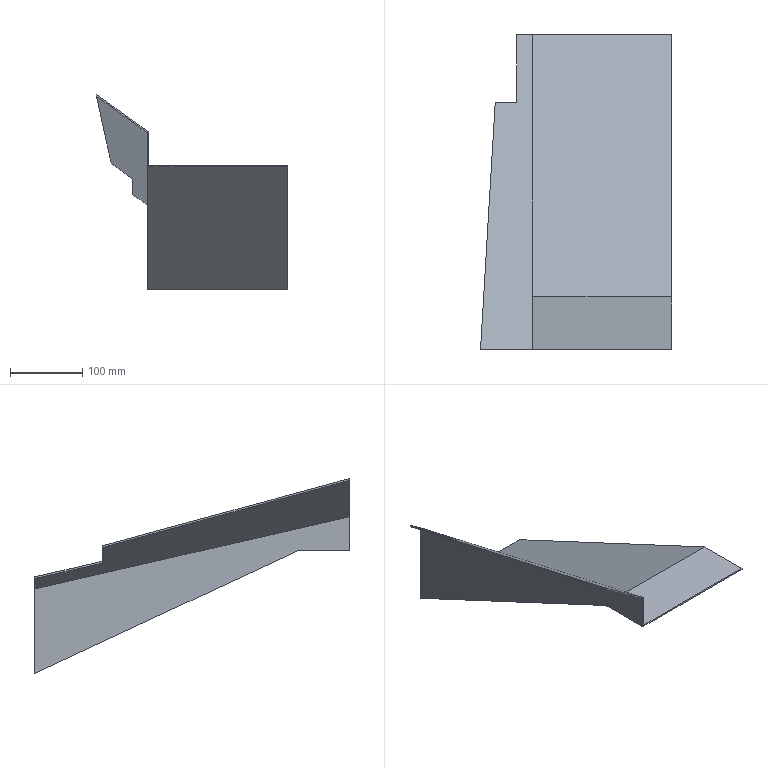Part | NX | features solid 2 | 1 solid | 14 faces | box 265.119 x 436.993 x 270.643 mm | volume 301955 mm3 | plane 13 | spline 1
STEP:
#1=CARTESIAN_POINT('',(815.34,325.702,-147.77));
#2=VERTEX_POINT('',#1);
#3=CARTESIAN_POINT('',(785.34,325.702,-126.218));
#4=VERTEX_POINT('',#3);
#5=CARTESIAN_POINT('',(723.013,325.702,-81.441));
#6=DIRECTION('',(0.8121,0.,-0.5835));
#7=VECTOR('',#6,1000.);
#8=LINE('',#5,#7);
#9=EDGE_CURVE('',#2,#4,#8,.F.);
#10=ORIENTED_EDGE('',*,*,#9,.F.);
#11=CARTESIAN_POINT('',(815.34,325.702,-150.275));
#12=VERTEX_POINT('',#11);
#13=CARTESIAN_POINT('',(815.34,325.702,-80.177));
#14=DIRECTION('',(0.,0.,-1.));
#15=VECTOR('',#14,1000.);
#16=LINE('',#13,#15);
#17=EDGE_CURVE('',#2,#12,#16,.T.);
#18=ORIENTED_EDGE('',*,*,#17,.T.);
#19=CARTESIAN_POINT('',(785.34,325.702,-128.723));
#20=VERTEX_POINT('',#19);
#21=CARTESIAN_POINT('',(721.826,325.702,-83.094));
#22=DIRECTION('',(0.8121,0.,-0.5835));
#23=VECTOR('',#22,1000.);
#24=LINE('',#21,#23);
#25=EDGE_CURVE('',#20,#12,#24,.T.);
#26=ORIENTED_EDGE('',*,*,#25,.F.);
#27=CARTESIAN_POINT('',(785.34,325.702,-80.177));
#28=DIRECTION('',(0.,0.,-1.));
#29=VECTOR('',#28,1000.);
#30=LINE('',#27,#29);
#31=EDGE_CURVE('',#4,#20,#30,.T.);
#32=ORIENTED_EDGE('',*,*,#31,.F.);
#33=EDGE_LOOP('',(#10,#18,#26,#32));
#34=FACE_BOUND('',#33,.T.);
#35=CARTESIAN_POINT('',(772.317,325.702,-80.177));
#36=DIRECTION('',(0.,-1.,0.));
#37=DIRECTION('',(0.,0.,-1.));
#38=AXIS2_PLACEMENT_3D('',#35,#36,#37);
#39=PLANE('',#38);
#40=ADVANCED_FACE('',(#34),#39,.F.);
#41=CARTESIAN_POINT('',(764.881,-17.,-32.884));
#42=VERTEX_POINT('',#41);
#43=CARTESIAN_POINT('',(837.317,-17.,-84.922));
#44=VERTEX_POINT('',#43);
#45=CARTESIAN_POINT('',(764.881,-17.,-32.884));
#46=CARTESIAN_POINT('',(789.026,-17.,-50.23));
#47=CARTESIAN_POINT('',(813.171,-17.,-67.576));
#48=CARTESIAN_POINT('',(837.317,-17.,-84.922));
#49=B_SPLINE_CURVE_WITH_KNOTS('',3,(#45,#46,#47,#48),.UNSPECIFIED.,.F.,.F.,(4,4),(-0.01905,0.07014),.UNSPECIFIED.);
#50=EDGE_CURVE('',#42,#44,#49,.T.);
#51=ORIENTED_EDGE('',*,*,#50,.F.);
#52=CARTESIAN_POINT('',(764.881,-17.,-35.389));
#53=VERTEX_POINT('',#52);
#54=CARTESIAN_POINT('',(764.881,-17.,-33.012));
#55=DIRECTION('',(0.,0.,1.));
#56=VECTOR('',#55,1000.);
#57=LINE('',#54,#56);
#58=EDGE_CURVE('',#42,#53,#57,.F.);
#59=ORIENTED_EDGE('',*,*,#58,.T.);
#60=CARTESIAN_POINT('',(835.317,-17.,-85.99));
#61=VERTEX_POINT('',#60);
#62=CARTESIAN_POINT('',(764.881,-17.,-35.389));
#63=CARTESIAN_POINT('',(788.359,-17.,-52.256));
#64=CARTESIAN_POINT('',(811.838,-17.,-69.123));
#65=CARTESIAN_POINT('',(835.317,-17.,-85.99));
#66=B_SPLINE_CURVE_WITH_KNOTS('',3,(#62,#63,#64,#65),.UNSPECIFIED.,.F.,.F.,(4,4),(-0.01764,0.06909),.UNSPECIFIED.);
#67=EDGE_CURVE('',#53,#61,#66,.T.);
#68=ORIENTED_EDGE('',*,*,#67,.T.);
#69=CARTESIAN_POINT('',(835.317,-17.,-133.495));
#70=VERTEX_POINT('',#69);
#71=CARTESIAN_POINT('',(835.317,-17.,-107.104));
#72=DIRECTION('',(0.,0.,1.));
#73=VECTOR('',#72,1000.);
#74=LINE('',#71,#73);
#75=EDGE_CURVE('',#70,#61,#74,.T.);
#76=ORIENTED_EDGE('',*,*,#75,.F.);
#77=CARTESIAN_POINT('',(1030.,-17.,-133.495));
#78=VERTEX_POINT('',#77);
#79=CARTESIAN_POINT('',(835.317,-17.,-133.495));
#80=CARTESIAN_POINT('',(900.211,-17.,-133.495));
#81=CARTESIAN_POINT('',(965.106,-17.,-133.495));
#82=CARTESIAN_POINT('',(1030.,-17.,-133.495));
#83=B_SPLINE_CURVE_WITH_KNOTS('',3,(#79,#80,#81,#82),.UNSPECIFIED.,.F.,.F.,(4,4),(0.,0.1947),.UNSPECIFIED.);
#84=EDGE_CURVE('',#70,#78,#83,.T.);
#85=ORIENTED_EDGE('',*,*,#84,.T.);
#86=CARTESIAN_POINT('',(1030.,-17.,-131.495));
#87=VERTEX_POINT('',#86);
#88=CARTESIAN_POINT('',(1030.,-17.,-132.495));
#89=DIRECTION('',(0.,0.,1.));
#90=VECTOR('',#89,1000.);
#91=LINE('',#88,#90);
#92=EDGE_CURVE('',#78,#87,#91,.T.);
#93=ORIENTED_EDGE('',*,*,#92,.T.);
#94=CARTESIAN_POINT('',(837.317,-17.,-131.495));
#95=VERTEX_POINT('',#94);
#96=CARTESIAN_POINT('',(837.317,-17.,-131.495));
#97=CARTESIAN_POINT('',(901.544,-17.,-131.495));
#98=CARTESIAN_POINT('',(965.772,-17.,-131.495));
#99=CARTESIAN_POINT('',(1030.,-17.,-131.495));
#100=B_SPLINE_CURVE_WITH_KNOTS('',3,(#96,#97,#98,#99),.UNSPECIFIED.,.F.,.F.,(4,4),(0.,0.1927),.UNSPECIFIED.);
#101=EDGE_CURVE('',#95,#87,#100,.T.);
#102=ORIENTED_EDGE('',*,*,#101,.F.);
#103=CARTESIAN_POINT('',(837.317,-17.,-105.57));
#104=DIRECTION('',(0.,0.,1.));
#105=VECTOR('',#104,1000.);
#106=LINE('',#103,#105);
#107=EDGE_CURVE('',#44,#95,#106,.F.);
#108=ORIENTED_EDGE('',*,*,#107,.F.);
#109=EDGE_LOOP('',(#51,#59,#68,#76,#85,#93,#102,#108));
#110=FACE_BOUND('',#109,.T.);
#111=CARTESIAN_POINT('',(1030.,-17.,-139.629));
#112=CARTESIAN_POINT('',(1030.,-17.,-42.536));
#113=CARTESIAN_POINT('',(1017.249,-17.,-139.629));
#114=CARTESIAN_POINT('',(1017.249,-17.,-42.536));
#115=CARTESIAN_POINT('',(991.747,-17.,-139.629));
#116=CARTESIAN_POINT('',(991.747,-17.,-42.536));
#117=CARTESIAN_POINT('',(959.87,-17.,-139.629));
#118=CARTESIAN_POINT('',(959.87,-17.,-42.536));
#119=CARTESIAN_POINT('',(934.368,-17.,-139.629));
#120=CARTESIAN_POINT('',(934.368,-17.,-42.536));
#121=CARTESIAN_POINT('',(915.241,-17.,-139.629));
#122=CARTESIAN_POINT('',(915.241,-17.,-42.536));
#123=CARTESIAN_POINT('',(896.115,-17.,-139.63));
#124=CARTESIAN_POINT('',(896.115,-17.,-42.537));
#125=CARTESIAN_POINT('',(880.175,-17.,-139.627));
#126=CARTESIAN_POINT('',(880.175,-17.,-42.533));
#127=CARTESIAN_POINT('',(869.02,-17.,-139.633));
#128=CARTESIAN_POINT('',(869.02,-17.,-42.539));
#129=CARTESIAN_POINT('',(862.641,-17.,-139.623));
#130=CARTESIAN_POINT('',(862.641,-17.,-42.53));
#131=CARTESIAN_POINT('',(857.869,-17.,-139.653));
#132=CARTESIAN_POINT('',(857.869,-17.,-42.559));
#133=CARTESIAN_POINT('',(853.037,-17.,-139.488));
#134=CARTESIAN_POINT('',(853.037,-17.,-42.395));
#135=CARTESIAN_POINT('',(848.214,-17.,-139.341));
#136=CARTESIAN_POINT('',(848.214,-17.,-42.248));
#137=CARTESIAN_POINT('',(843.577,-17.,-139.83));
#138=CARTESIAN_POINT('',(843.577,-17.,-42.737));
#139=CARTESIAN_POINT('',(839.137,-17.,-141.121));
#140=CARTESIAN_POINT('',(839.137,-17.,-44.028));
#141=CARTESIAN_POINT('',(834.715,-17.,-142.775));
#142=CARTESIAN_POINT('',(834.715,-17.,-45.682));
#143=CARTESIAN_POINT('',(828.593,-17.,-144.624));
#144=CARTESIAN_POINT('',(828.593,-17.,-47.531));
#145=CARTESIAN_POINT('',(820.431,-17.,-144.906));
#146=CARTESIAN_POINT('',(820.431,-17.,-47.812));
#147=CARTESIAN_POINT('',(812.873,-17.,-142.36));
#148=CARTESIAN_POINT('',(812.873,-17.,-45.267));
#149=CARTESIAN_POINT('',(807.015,-17.,-140.172));
#150=CARTESIAN_POINT('',(807.015,-17.,-43.079));
#151=CARTESIAN_POINT('',(801.031,-17.,-138.263));
#152=CARTESIAN_POINT('',(801.031,-17.,-41.17));
#153=CARTESIAN_POINT('',(793.243,-17.,-136.384));
#154=CARTESIAN_POINT('',(793.243,-17.,-39.291));
#155=CARTESIAN_POINT('',(784.909,-17.,-131.641));
#156=CARTESIAN_POINT('',(784.909,-17.,-34.548));
#157=CARTESIAN_POINT('',(778.905,-17.,-123.694));
#158=CARTESIAN_POINT('',(778.905,-17.,-26.601));
#159=CARTESIAN_POINT('',(775.672,-17.,-116.308));
#160=CARTESIAN_POINT('',(775.672,-17.,-19.215));
#161=CARTESIAN_POINT('',(773.734,-17.,-110.553));
#162=CARTESIAN_POINT('',(773.734,-17.,-13.459));
#163=CARTESIAN_POINT('',(772.653,-17.,-106.122));
#164=CARTESIAN_POINT('',(772.653,-17.,-9.029));
#165=CARTESIAN_POINT('',(772.039,-17.,-101.297));
#166=CARTESIAN_POINT('',(772.039,-17.,-4.204));
#167=CARTESIAN_POINT('',(771.795,-17.,-94.179));
#168=CARTESIAN_POINT('',(771.795,-17.,2.914));
#169=CARTESIAN_POINT('',(771.535,-17.,-86.911));
#170=CARTESIAN_POINT('',(771.535,-17.,10.182));
#171=CARTESIAN_POINT('',(768.627,-17.,-82.777));
#172=CARTESIAN_POINT('',(768.627,-17.,14.316));
#173=CARTESIAN_POINT('',(766.237,-17.,-81.837));
#174=CARTESIAN_POINT('',(766.237,-17.,15.257));
#175=CARTESIAN_POINT('',(764.881,-17.,-81.558));
#176=CARTESIAN_POINT('',(764.881,-17.,15.535));
#177=B_SPLINE_SURFACE_WITH_KNOTS('',3,1,((#111,#112),(#113,#114),(#115,#116),(#117,#118),(#119,#120),(#121,#122),(#123,#124),(#125,#126),(#127,#128),(#129,#130),(#131,#132),(#133,#134),(#135,#136),(#137,#138),(#139,#140),(#141,#142),(#143,#144),(#145,#146),(#147,#148),(#149,#150),(#151,#152),(#153,#154),(#155,#156),(#157,#158),(#159,#160),(#161,#162),(#163,#164),(#165,#166),(#167,#168),(#169,#170),(#171,#172),(#173,#174),(#175,#176)),.SURF_OF_LINEAR_EXTRUSION.,.F.,.F.,.F.,(4,1,1,1,1,1,1,1,1,1,1,1,1,1,1,1,1,1,1,1,1,1,1,1,1,1,1,1,1,1,4),(2,2),(-1.184,-0.9175,-0.6509,-0.5176,-0.3843,-0.251,-0.1177,-0.051,-0.01768,0.01565,0.04898,0.08231,0.1156,0.149,0.1823,0.2156,0.2823,0.3489,0.3823,0.4156,0.4822,0.5489,0.6155,0.6822,0.7155,0.7489,0.7822,0.8155,0.8822,0.9155,0.9488),(0.,1.),.UNSPECIFIED.);
#178=ADVANCED_FACE('',(#110),#177,.F.);
#179=ORIENTED_EDGE('',*,*,#50,.T.);
#180=CARTESIAN_POINT('',(837.317,419.993,-185.194));
#181=VERTEX_POINT('',#180);
#182=CARTESIAN_POINT('',(837.317,418.909,-184.945));
#183=DIRECTION('',(0.,0.9747,-0.2236));
#184=VECTOR('',#183,1000.);
#185=LINE('',#182,#184);
#186=EDGE_CURVE('',#181,#44,#185,.F.);
#187=ORIENTED_EDGE('',*,*,#186,.F.);
#188=CARTESIAN_POINT('',(815.34,419.993,-169.406));
#189=VERTEX_POINT('',#188);
#190=CARTESIAN_POINT('',(792.078,419.993,-152.694));
#191=DIRECTION('',(-0.8121,0.,0.5835));
#192=VECTOR('',#191,1000.);
#193=LINE('',#190,#192);
#194=EDGE_CURVE('',#181,#189,#193,.T.);
#195=ORIENTED_EDGE('',*,*,#194,.T.);
#196=CARTESIAN_POINT('',(815.34,349.955,-153.335));
#197=DIRECTION('',(0.,0.9747,-0.2236));
#198=VECTOR('',#197,1000.);
#199=LINE('',#196,#198);
#200=EDGE_CURVE('',#189,#2,#199,.F.);
#201=ORIENTED_EDGE('',*,*,#200,.T.);
#202=ORIENTED_EDGE('',*,*,#9,.T.);
#203=CARTESIAN_POINT('',(790.938,419.454,-151.751));
#204=DIRECTION('',(-0.05751,-0.9633,0.2623));
#205=VECTOR('',#204,1000.);
#206=LINE('',#203,#205);
#207=EDGE_CURVE('',#42,#4,#206,.F.);
#208=ORIENTED_EDGE('',*,*,#207,.F.);
#209=EDGE_LOOP('',(#179,#187,#195,#201,#202,#208));
#210=FACE_BOUND('',#209,.T.);
#211=CARTESIAN_POINT('',(710.723,438.733,-98.548));
#212=DIRECTION('',(0.5736,0.1832,0.7984));
#213=DIRECTION('',(-0.1552,0.9813,-0.1137));
#214=AXIS2_PLACEMENT_3D('',#211,#212,#213);
#215=PLANE('',#214);
#216=ADVANCED_FACE('',(#210),#215,.T.);
#217=ORIENTED_EDGE('',*,*,#25,.T.);
#218=CARTESIAN_POINT('',(815.34,419.993,-171.911));
#219=VERTEX_POINT('',#218);
#220=CARTESIAN_POINT('',(815.34,421.804,-172.326));
#221=DIRECTION('',(0.,-0.9747,0.2236));
#222=VECTOR('',#221,1000.);
#223=LINE('',#220,#222);
#224=EDGE_CURVE('',#219,#12,#223,.T.);
#225=ORIENTED_EDGE('',*,*,#224,.F.);
#226=CARTESIAN_POINT('',(835.317,419.993,-186.262));
#227=VERTEX_POINT('',#226);
#228=CARTESIAN_POINT('',(790.891,419.993,-154.346));
#229=DIRECTION('',(0.8121,0.,-0.5835));
#230=VECTOR('',#229,1000.);
#231=LINE('',#228,#230);
#232=EDGE_CURVE('',#219,#227,#231,.T.);
#233=ORIENTED_EDGE('',*,*,#232,.T.);
#234=CARTESIAN_POINT('',(835.317,322.751,-163.949));
#235=DIRECTION('',(0.,-0.9747,0.2236));
#236=VECTOR('',#235,1000.);
#237=LINE('',#234,#236);
#238=EDGE_CURVE('',#227,#61,#237,.T.);
#239=ORIENTED_EDGE('',*,*,#238,.T.);
#240=ORIENTED_EDGE('',*,*,#67,.F.);
#241=CARTESIAN_POINT('',(790.9,418.821,-154.084));
#242=DIRECTION('',(-0.05751,-0.9633,0.2623));
#243=VECTOR('',#242,1000.);
#244=LINE('',#241,#243);
#245=EDGE_CURVE('',#20,#53,#244,.T.);
#246=ORIENTED_EDGE('',*,*,#245,.F.);
#247=EDGE_LOOP('',(#217,#225,#233,#239,#240,#246));
#248=FACE_BOUND('',#247,.T.);
#249=CARTESIAN_POINT('',(709.576,438.367,-100.145));
#250=DIRECTION('',(0.5736,0.1832,0.7984));
#251=DIRECTION('',(-0.1552,0.9813,-0.1137));
#252=AXIS2_PLACEMENT_3D('',#249,#250,#251);
#253=PLANE('',#252);
#254=ADVANCED_FACE('',(#248),#253,.F.);
#255=CARTESIAN_POINT('',(1030.,419.993,-301.319));
#256=VERTEX_POINT('',#255);
#257=CARTESIAN_POINT('',(1030.,55.804,-131.495));
#258=VERTEX_POINT('',#257);
#259=CARTESIAN_POINT('',(1030.,442.654,-311.886));
#260=DIRECTION('',(0.,-0.9063,0.4226));
#261=VECTOR('',#260,1000.);
#262=LINE('',#259,#261);
#263=EDGE_CURVE('',#256,#258,#262,.T.);
#264=ORIENTED_EDGE('',*,*,#263,.F.);
#265=CARTESIAN_POINT('',(837.317,419.993,-301.319));
#266=VERTEX_POINT('',#265);
#267=CARTESIAN_POINT('',(747.317,419.993,-301.319));
#268=DIRECTION('',(1.,0.,0.));
#269=VECTOR('',#268,1000.);
#270=LINE('',#267,#269);
#271=EDGE_CURVE('',#256,#266,#270,.F.);
#272=ORIENTED_EDGE('',*,*,#271,.T.);
#273=CARTESIAN_POINT('',(837.317,55.804,-131.495));
#274=VERTEX_POINT('',#273);
#275=CARTESIAN_POINT('',(837.317,442.654,-311.886));
#276=DIRECTION('',(0.,-0.9063,0.4226));
#277=VECTOR('',#276,1000.);
#278=LINE('',#275,#277);
#279=EDGE_CURVE('',#266,#274,#278,.T.);
#280=ORIENTED_EDGE('',*,*,#279,.T.);
#281=CARTESIAN_POINT('',(930.,55.804,-131.495));
#282=DIRECTION('',(-1.,0.,0.));
#283=VECTOR('',#282,1000.);
#284=LINE('',#281,#283);
#285=EDGE_CURVE('',#258,#274,#284,.T.);
#286=ORIENTED_EDGE('',*,*,#285,.F.);
#287=EDGE_LOOP('',(#264,#272,#280,#286));
#288=FACE_BOUND('',#287,.T.);
#289=CARTESIAN_POINT('',(930.,442.654,-311.886));
#290=DIRECTION('',(0.,-0.4226,-0.9063));
#291=DIRECTION('',(1.,0.,0.));
#292=AXIS2_PLACEMENT_3D('',#289,#290,#291);
#293=PLANE('',#292);
#294=ADVANCED_FACE('',(#288),#293,.F.);
#295=CARTESIAN_POINT('',(1030.,419.993,-303.526));
#296=VERTEX_POINT('',#295);
#297=CARTESIAN_POINT('',(1030.,55.36,-133.495));
#298=VERTEX_POINT('',#297);
#299=CARTESIAN_POINT('',(1030.,441.809,-313.699));
#300=DIRECTION('',(0.,-0.9063,0.4226));
#301=VECTOR('',#300,1000.);
#302=LINE('',#299,#301);
#303=EDGE_CURVE('',#296,#298,#302,.T.);
#304=ORIENTED_EDGE('',*,*,#303,.F.);
#305=CARTESIAN_POINT('',(1030.,419.993,-125.));
#306=DIRECTION('',(0.,0.,-1.));
#307=VECTOR('',#306,1000.);
#308=LINE('',#305,#307);
#309=EDGE_CURVE('',#296,#256,#308,.F.);
#310=ORIENTED_EDGE('',*,*,#309,.T.);
#311=ORIENTED_EDGE('',*,*,#263,.T.);
#312=CARTESIAN_POINT('',(1030.,-55.,-131.495));
#313=DIRECTION('',(0.,1.,0.));
#314=VECTOR('',#313,1000.);
#315=LINE('',#312,#314);
#316=EDGE_CURVE('',#87,#258,#315,.T.);
#317=ORIENTED_EDGE('',*,*,#316,.F.);
#318=ORIENTED_EDGE('',*,*,#92,.F.);
#319=CARTESIAN_POINT('',(1030.,-55.,-133.495));
#320=DIRECTION('',(0.,1.,0.));
#321=VECTOR('',#320,1000.);
#322=LINE('',#319,#321);
#323=EDGE_CURVE('',#78,#298,#322,.T.);
#324=ORIENTED_EDGE('',*,*,#323,.T.);
#325=EDGE_LOOP('',(#304,#310,#311,#317,#318,#324));
#326=FACE_BOUND('',#325,.T.);
#327=CARTESIAN_POINT('',(1030.,-575.,-125.));
#328=DIRECTION('',(1.,0.,0.));
#329=DIRECTION('',(0.,0.,-1.));
#330=AXIS2_PLACEMENT_3D('',#327,#328,#329);
#331=PLANE('',#330);
#332=ADVANCED_FACE('',(#326),#331,.T.);
#333=CARTESIAN_POINT('',(835.317,419.993,-303.526));
#334=VERTEX_POINT('',#333);
#335=CARTESIAN_POINT('',(835.317,55.36,-133.495));
#336=VERTEX_POINT('',#335);
#337=CARTESIAN_POINT('',(835.317,300.974,-248.027));
#338=DIRECTION('',(0.,0.9063,-0.4226));
#339=VECTOR('',#338,1000.);
#340=LINE('',#337,#339);
#341=EDGE_CURVE('',#334,#336,#340,.F.);
#342=ORIENTED_EDGE('',*,*,#341,.F.);
#343=CARTESIAN_POINT('',(747.317,419.993,-303.526));
#344=DIRECTION('',(1.,0.,0.));
#345=VECTOR('',#344,1000.);
#346=LINE('',#343,#345);
#347=EDGE_CURVE('',#296,#334,#346,.F.);
#348=ORIENTED_EDGE('',*,*,#347,.F.);
#349=ORIENTED_EDGE('',*,*,#303,.T.);
#350=CARTESIAN_POINT('',(778.845,55.36,-133.495));
#351=DIRECTION('',(1.,0.,0.));
#352=VECTOR('',#351,1000.);
#353=LINE('',#350,#352);
#354=EDGE_CURVE('',#336,#298,#353,.T.);
#355=ORIENTED_EDGE('',*,*,#354,.F.);
#356=EDGE_LOOP('',(#342,#348,#349,#355));
#357=FACE_BOUND('',#356,.T.);
#358=CARTESIAN_POINT('',(930.,441.809,-313.699));
#359=DIRECTION('',(0.,-0.4226,-0.9063));
#360=DIRECTION('',(1.,0.,0.));
#361=AXIS2_PLACEMENT_3D('',#358,#359,#360);
#362=PLANE('',#361);
#363=ADVANCED_FACE('',(#357),#362,.T.);
#364=CARTESIAN_POINT('',(837.317,-80.,-131.495));
#365=DIRECTION('',(0.,-1.,0.));
#366=VECTOR('',#365,1000.);
#367=LINE('',#364,#366);
#368=EDGE_CURVE('',#95,#274,#367,.F.);
#369=ORIENTED_EDGE('',*,*,#368,.F.);
#370=ORIENTED_EDGE('',*,*,#101,.T.);
#371=ORIENTED_EDGE('',*,*,#316,.T.);
#372=ORIENTED_EDGE('',*,*,#285,.T.);
#373=EDGE_LOOP('',(#369,#370,#371,#372));
#374=FACE_BOUND('',#373,.T.);
#375=CARTESIAN_POINT('',(778.845,-55.,-131.495));
#376=DIRECTION('',(0.,0.,1.));
#377=DIRECTION('',(1.,0.,0.));
#378=AXIS2_PLACEMENT_3D('',#375,#376,#377);
#379=PLANE('',#378);
#380=ADVANCED_FACE('',(#374),#379,.T.);
#381=ORIENTED_EDGE('',*,*,#84,.F.);
#382=CARTESIAN_POINT('',(835.317,305.865,-133.495));
#383=DIRECTION('',(0.,-1.,0.));
#384=VECTOR('',#383,1000.);
#385=LINE('',#382,#384);
#386=EDGE_CURVE('',#70,#336,#385,.F.);
#387=ORIENTED_EDGE('',*,*,#386,.T.);
#388=ORIENTED_EDGE('',*,*,#354,.T.);
#389=ORIENTED_EDGE('',*,*,#323,.F.);
#390=EDGE_LOOP('',(#381,#387,#388,#389));
#391=FACE_BOUND('',#390,.T.);
#392=CARTESIAN_POINT('',(778.845,-55.,-133.495));
#393=DIRECTION('',(0.,0.,1.));
#394=DIRECTION('',(1.,0.,0.));
#395=AXIS2_PLACEMENT_3D('',#392,#393,#394);
#396=PLANE('',#395);
#397=ADVANCED_FACE('',(#391),#396,.F.);
#398=ORIENTED_EDGE('',*,*,#279,.F.);
#399=CARTESIAN_POINT('',(837.317,419.993,-237.54));
#400=DIRECTION('',(0.,0.,-1.));
#401=VECTOR('',#400,1000.);
#402=LINE('',#399,#401);
#403=EDGE_CURVE('',#266,#181,#402,.F.);
#404=ORIENTED_EDGE('',*,*,#403,.T.);
#405=ORIENTED_EDGE('',*,*,#186,.T.);
#406=ORIENTED_EDGE('',*,*,#107,.T.);
#407=ORIENTED_EDGE('',*,*,#368,.T.);
#408=EDGE_LOOP('',(#398,#404,#405,#406,#407));
#409=FACE_BOUND('',#408,.T.);
#410=CARTESIAN_POINT('',(837.317,305.865,-237.54));
#411=DIRECTION('',(1.,0.,0.));
#412=DIRECTION('',(0.,1.,0.));
#413=AXIS2_PLACEMENT_3D('',#410,#411,#412);
#414=PLANE('',#413);
#415=ADVANCED_FACE('',(#409),#414,.T.);
#416=ORIENTED_EDGE('',*,*,#238,.F.);
#417=CARTESIAN_POINT('',(835.317,419.993,-237.54));
#418=DIRECTION('',(0.,0.,-1.));
#419=VECTOR('',#418,1000.);
#420=LINE('',#417,#419);
#421=EDGE_CURVE('',#334,#227,#420,.F.);
#422=ORIENTED_EDGE('',*,*,#421,.F.);
#423=ORIENTED_EDGE('',*,*,#341,.T.);
#424=ORIENTED_EDGE('',*,*,#386,.F.);
#425=ORIENTED_EDGE('',*,*,#75,.T.);
#426=EDGE_LOOP('',(#416,#422,#423,#424,#425));
#427=FACE_BOUND('',#426,.T.);
#428=CARTESIAN_POINT('',(835.317,305.865,-237.54));
#429=DIRECTION('',(1.,0.,0.));
#430=DIRECTION('',(0.,1.,0.));
#431=AXIS2_PLACEMENT_3D('',#428,#429,#430);
#432=PLANE('',#431);
#433=ADVANCED_FACE('',(#427),#432,.F.);
#434=ORIENTED_EDGE('',*,*,#421,.T.);
#435=ORIENTED_EDGE('',*,*,#232,.F.);
#436=CARTESIAN_POINT('',(815.34,419.993,-89.123));
#437=DIRECTION('',(0.,0.,1.));
#438=VECTOR('',#437,1000.);
#439=LINE('',#436,#438);
#440=EDGE_CURVE('',#189,#219,#439,.F.);
#441=ORIENTED_EDGE('',*,*,#440,.F.);
#442=ORIENTED_EDGE('',*,*,#194,.F.);
#443=ORIENTED_EDGE('',*,*,#403,.F.);
#444=ORIENTED_EDGE('',*,*,#271,.F.);
#445=ORIENTED_EDGE('',*,*,#309,.F.);
#446=ORIENTED_EDGE('',*,*,#347,.T.);
#447=EDGE_LOOP('',(#434,#435,#441,#442,#443,#444,#445,#446));
#448=FACE_BOUND('',#447,.T.);
#449=CARTESIAN_POINT('',(747.317,419.993,-215.));
#450=DIRECTION('',(0.,-1.,0.));
#451=DIRECTION('',(1.,0.,0.));
#452=AXIS2_PLACEMENT_3D('',#449,#450,#451);
#453=PLANE('',#452);
#454=ADVANCED_FACE('',(#448),#453,.F.);
#455=ORIENTED_EDGE('',*,*,#58,.F.);
#456=ORIENTED_EDGE('',*,*,#207,.T.);
#457=ORIENTED_EDGE('',*,*,#31,.T.);
#458=ORIENTED_EDGE('',*,*,#245,.T.);
#459=EDGE_LOOP('',(#455,#456,#457,#458));
#460=FACE_BOUND('',#459,.T.);
#461=CARTESIAN_POINT('',(763.264,-44.075,0.));
#462=DIRECTION('',(-0.9982,0.0596,0.));
#463=DIRECTION('',(-0.0596,-0.9982,0.));
#464=AXIS2_PLACEMENT_3D('',#461,#462,#463);
#465=PLANE('',#464);
#466=ADVANCED_FACE('',(#460),#465,.T.);
#467=ORIENTED_EDGE('',*,*,#17,.F.);
#468=ORIENTED_EDGE('',*,*,#200,.F.);
#469=ORIENTED_EDGE('',*,*,#440,.T.);
#470=ORIENTED_EDGE('',*,*,#224,.T.);
#471=EDGE_LOOP('',(#467,#468,#469,#470));
#472=FACE_BOUND('',#471,.T.);
#473=CARTESIAN_POINT('',(815.34,364.689,-89.123));
#474=DIRECTION('',(-1.,0.,0.));
#475=DIRECTION('',(0.,-1.,0.));
#476=AXIS2_PLACEMENT_3D('',#473,#474,#475);
#477=PLANE('',#476);
#478=ADVANCED_FACE('',(#472),#477,.T.);
#479=CLOSED_SHELL('',(#40,#178,#216,#254,#294,#332,#363,#380,#397,#415,#433,#454,#466,#478));
#480=MANIFOLD_SOLID_BREP('',#479);
#481=(LENGTH_UNIT()NAMED_UNIT(*)SI_UNIT(.MILLI.,.METRE.));
#482=UNCERTAINTY_MEASURE_WITH_UNIT(LENGTH_MEASURE(0.0508),#481,'','');
#483=(NAMED_UNIT(*)PLANE_ANGLE_UNIT()SI_UNIT($,.RADIAN.));
#484=(NAMED_UNIT(*)SI_UNIT($,.STERADIAN.)SOLID_ANGLE_UNIT());
#485=(GEOMETRIC_REPRESENTATION_CONTEXT(3)GLOBAL_UNCERTAINTY_ASSIGNED_CONTEXT((#482))GLOBAL_UNIT_ASSIGNED_CONTEXT((#481,#483,#484))REPRESENTATION_CONTEXT('',''));
#486=ADVANCED_BREP_SHAPE_REPRESENTATION('',(#480),#485);